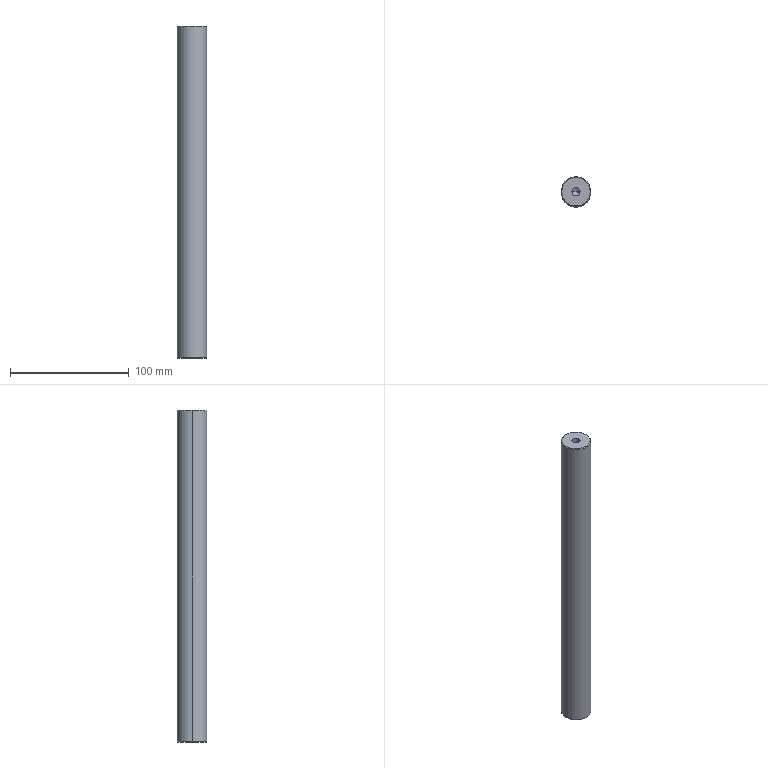Part | SolidWorks | features HoleWzd 2, Chamfer 1, Extrusion 1 | 1 solid | 16 faces | box 25 x 25 x 280 mm | volume 135760 mm3 | cone 8 | cylinder 6 | plane 2 | commonest cylinder face diameters 6.8 x4 25 x2
STEP:
#1=CARTESIAN_POINT('',(-12.,0.,0.));
#2=VERTEX_POINT('',#1);
#3=CARTESIAN_POINT('',(12.,0.,0.));
#4=VERTEX_POINT('',#3);
#5=CARTESIAN_POINT('',(0.,0.,0.));
#6=DIRECTION('',(0.,0.,-1.));
#7=DIRECTION('',(1.,0.,0.));
#8=AXIS2_PLACEMENT_3D('',#5,#6,#7);
#9=CIRCLE('',#8,12.);
#10=EDGE_CURVE('',#2,#4,#9,.T.);
#11=ORIENTED_EDGE('',*,*,#10,.F.);
#12=CARTESIAN_POINT('',(-12.5,0.,0.5));
#13=VERTEX_POINT('',#12);
#14=CARTESIAN_POINT('',(-12.5,0.,0.5));
#15=DIRECTION('',(-0.7071,0.,0.7071));
#16=VECTOR('',#15,1000.);
#17=LINE('',#14,#16);
#18=EDGE_CURVE('',#2,#13,#17,.T.);
#19=ORIENTED_EDGE('',*,*,#18,.T.);
#20=CARTESIAN_POINT('',(12.5,0.,0.5));
#21=VERTEX_POINT('',#20);
#22=CARTESIAN_POINT('',(0.,0.,0.5));
#23=DIRECTION('',(0.,0.,1.));
#24=DIRECTION('',(1.,0.,0.));
#25=AXIS2_PLACEMENT_3D('',#22,#23,#24);
#26=CIRCLE('',#25,12.5);
#27=EDGE_CURVE('',#21,#13,#26,.T.);
#28=ORIENTED_EDGE('',*,*,#27,.F.);
#29=CARTESIAN_POINT('',(12.5,0.,0.5));
#30=DIRECTION('',(0.7071,0.,0.7071));
#31=VECTOR('',#30,1000.);
#32=LINE('',#29,#31);
#33=EDGE_CURVE('',#4,#21,#32,.T.);
#34=ORIENTED_EDGE('',*,*,#33,.F.);
#35=EDGE_LOOP('',(#11,#19,#28,#34));
#36=FACE_OUTER_BOUND('',#35,.T.);
#37=CARTESIAN_POINT('',(0.,0.,0.5));
#38=DIRECTION('',(0.,0.,1.));
#39=DIRECTION('',(1.,0.,0.));
#40=AXIS2_PLACEMENT_3D('',#37,#38,#39);
#41=CONICAL_SURFACE('',#40,12.5,0.7854);
#42=ADVANCED_FACE('',(#36),#41,.T.);
#43=CARTESIAN_POINT('',(12.,0.,280.));
#44=VERTEX_POINT('',#43);
#45=CARTESIAN_POINT('',(-12.,0.,280.));
#46=VERTEX_POINT('',#45);
#47=CARTESIAN_POINT('',(0.,0.,280.));
#48=DIRECTION('',(0.,0.,1.));
#49=DIRECTION('',(1.,0.,0.));
#50=AXIS2_PLACEMENT_3D('',#47,#48,#49);
#51=CIRCLE('',#50,12.);
#52=EDGE_CURVE('',#44,#46,#51,.T.);
#53=ORIENTED_EDGE('',*,*,#52,.F.);
#54=CARTESIAN_POINT('',(12.5,0.,279.5));
#55=VERTEX_POINT('',#54);
#56=CARTESIAN_POINT('',(12.,0.,280.));
#57=DIRECTION('',(0.7071,0.,-0.7071));
#58=VECTOR('',#57,1000.);
#59=LINE('',#56,#58);
#60=EDGE_CURVE('',#44,#55,#59,.T.);
#61=ORIENTED_EDGE('',*,*,#60,.T.);
#62=CARTESIAN_POINT('',(-12.5,0.,279.5));
#63=VERTEX_POINT('',#62);
#64=CARTESIAN_POINT('',(0.,0.,279.5));
#65=DIRECTION('',(0.,0.,-1.));
#66=DIRECTION('',(1.,0.,0.));
#67=AXIS2_PLACEMENT_3D('',#64,#65,#66);
#68=CIRCLE('',#67,12.5);
#69=EDGE_CURVE('',#63,#55,#68,.T.);
#70=ORIENTED_EDGE('',*,*,#69,.F.);
#71=CARTESIAN_POINT('',(-12.,0.,280.));
#72=DIRECTION('',(-0.7071,0.,-0.7071));
#73=VECTOR('',#72,1000.);
#74=LINE('',#71,#73);
#75=EDGE_CURVE('',#46,#63,#74,.T.);
#76=ORIENTED_EDGE('',*,*,#75,.F.);
#77=EDGE_LOOP('',(#53,#61,#70,#76));
#78=FACE_OUTER_BOUND('',#77,.T.);
#79=CARTESIAN_POINT('',(0.,0.,280.));
#80=DIRECTION('',(0.,0.,-1.));
#81=DIRECTION('',(-1.,0.,0.));
#82=AXIS2_PLACEMENT_3D('',#79,#80,#81);
#83=CONICAL_SURFACE('',#82,12.,0.7854);
#84=ADVANCED_FACE('',(#78),#83,.T.);
#85=CARTESIAN_POINT('',(3.4,0.,22.25));
#86=VERTEX_POINT('',#85);
#87=CARTESIAN_POINT('',(-3.4,0.,22.25));
#88=VERTEX_POINT('',#87);
#89=CARTESIAN_POINT('',(0.,0.,22.25));
#90=DIRECTION('',(0.,0.,-1.));
#91=DIRECTION('',(-1.,0.,0.));
#92=AXIS2_PLACEMENT_3D('',#89,#90,#91);
#93=CIRCLE('',#92,3.4);
#94=EDGE_CURVE('',#86,#88,#93,.T.);
#95=ORIENTED_EDGE('',*,*,#94,.F.);
#96=CARTESIAN_POINT('',(3.4,0.,0.));
#97=VERTEX_POINT('',#96);
#98=CARTESIAN_POINT('',(3.4,0.,0.));
#99=DIRECTION('',(0.,0.,-1.));
#100=VECTOR('',#99,1000.);
#101=LINE('',#98,#100);
#102=EDGE_CURVE('',#86,#97,#101,.T.);
#103=ORIENTED_EDGE('',*,*,#102,.T.);
#104=CARTESIAN_POINT('',(-3.4,0.,0.));
#105=VERTEX_POINT('',#104);
#106=CARTESIAN_POINT('',(0.,0.,0.));
#107=DIRECTION('',(0.,0.,-1.));
#108=DIRECTION('',(-1.,0.,0.));
#109=AXIS2_PLACEMENT_3D('',#106,#107,#108);
#110=CIRCLE('',#109,3.4);
#111=EDGE_CURVE('',#97,#105,#110,.T.);
#112=ORIENTED_EDGE('',*,*,#111,.T.);
#113=CARTESIAN_POINT('',(-3.4,0.,0.));
#114=DIRECTION('',(0.,0.,-1.));
#115=VECTOR('',#114,1000.);
#116=LINE('',#113,#115);
#117=EDGE_CURVE('',#88,#105,#116,.T.);
#118=ORIENTED_EDGE('',*,*,#117,.F.);
#119=EDGE_LOOP('',(#95,#103,#112,#118));
#120=FACE_OUTER_BOUND('',#119,.T.);
#121=CARTESIAN_POINT('',(0.,0.,0.));
#122=DIRECTION('',(0.,0.,-1.));
#123=DIRECTION('',(-1.,0.,0.));
#124=AXIS2_PLACEMENT_3D('',#121,#122,#123);
#125=CYLINDRICAL_SURFACE('',#124,3.4);
#126=ADVANCED_FACE('',(#120),#125,.F.);
#127=CARTESIAN_POINT('',(0.,0.,24.293));
#128=VERTEX_POINT('',#127);
#129=CARTESIAN_POINT('',(-3.4,0.,22.25));
#130=DIRECTION('',(-0.8572,0.,-0.515));
#131=VECTOR('',#130,1000.);
#132=LINE('',#129,#131);
#133=EDGE_CURVE('',#128,#88,#132,.T.);
#134=ORIENTED_EDGE('',*,*,#133,.F.);
#135=CARTESIAN_POINT('',(3.4,0.,22.25));
#136=DIRECTION('',(0.8572,0.,-0.515));
#137=VECTOR('',#136,1000.);
#138=LINE('',#135,#137);
#139=EDGE_CURVE('',#128,#86,#138,.T.);
#140=ORIENTED_EDGE('',*,*,#139,.T.);
#141=ORIENTED_EDGE('',*,*,#94,.T.);
#142=EDGE_LOOP('',(#134,#140,#141));
#143=FACE_OUTER_BOUND('',#142,.T.);
#144=CARTESIAN_POINT('',(0.,0.,22.25));
#145=DIRECTION('',(0.,0.,-1.));
#146=DIRECTION('',(-1.,0.,0.));
#147=AXIS2_PLACEMENT_3D('',#144,#145,#146);
#148=CONICAL_SURFACE('',#147,3.4,1.03);
#149=ADVANCED_FACE('',(#143),#148,.F.);
#150=CARTESIAN_POINT('',(-3.4,0.,257.75));
#151=VERTEX_POINT('',#150);
#152=CARTESIAN_POINT('',(3.4,0.,257.75));
#153=VERTEX_POINT('',#152);
#154=CARTESIAN_POINT('',(0.,0.,257.75));
#155=DIRECTION('',(0.,0.,1.));
#156=DIRECTION('',(1.,0.,0.));
#157=AXIS2_PLACEMENT_3D('',#154,#155,#156);
#158=CIRCLE('',#157,3.4);
#159=EDGE_CURVE('',#151,#153,#158,.T.);
#160=ORIENTED_EDGE('',*,*,#159,.F.);
#161=CARTESIAN_POINT('',(-3.4,0.,280.));
#162=VERTEX_POINT('',#161);
#163=CARTESIAN_POINT('',(-3.4,0.,280.));
#164=DIRECTION('',(0.,0.,1.));
#165=VECTOR('',#164,1000.);
#166=LINE('',#163,#165);
#167=EDGE_CURVE('',#151,#162,#166,.T.);
#168=ORIENTED_EDGE('',*,*,#167,.T.);
#169=CARTESIAN_POINT('',(3.4,0.,280.));
#170=VERTEX_POINT('',#169);
#171=CARTESIAN_POINT('',(0.,0.,280.));
#172=DIRECTION('',(0.,0.,1.));
#173=DIRECTION('',(1.,0.,0.));
#174=AXIS2_PLACEMENT_3D('',#171,#172,#173);
#175=CIRCLE('',#174,3.4);
#176=EDGE_CURVE('',#162,#170,#175,.T.);
#177=ORIENTED_EDGE('',*,*,#176,.T.);
#178=CARTESIAN_POINT('',(3.4,0.,280.));
#179=DIRECTION('',(0.,0.,1.));
#180=VECTOR('',#179,1000.);
#181=LINE('',#178,#180);
#182=EDGE_CURVE('',#153,#170,#181,.T.);
#183=ORIENTED_EDGE('',*,*,#182,.F.);
#184=EDGE_LOOP('',(#160,#168,#177,#183));
#185=FACE_OUTER_BOUND('',#184,.T.);
#186=CARTESIAN_POINT('',(0.,0.,280.));
#187=DIRECTION('',(0.,0.,1.));
#188=DIRECTION('',(1.,0.,0.));
#189=AXIS2_PLACEMENT_3D('',#186,#187,#188);
#190=CYLINDRICAL_SURFACE('',#189,3.4);
#191=ADVANCED_FACE('',(#185),#190,.F.);
#192=CARTESIAN_POINT('',(0.,0.,255.707));
#193=VERTEX_POINT('',#192);
#194=CARTESIAN_POINT('',(3.4,0.,257.75));
#195=DIRECTION('',(0.8572,0.,0.515));
#196=VECTOR('',#195,1000.);
#197=LINE('',#194,#196);
#198=EDGE_CURVE('',#193,#153,#197,.T.);
#199=ORIENTED_EDGE('',*,*,#198,.F.);
#200=CARTESIAN_POINT('',(-3.4,0.,257.75));
#201=DIRECTION('',(-0.8572,0.,0.515));
#202=VECTOR('',#201,1000.);
#203=LINE('',#200,#202);
#204=EDGE_CURVE('',#193,#151,#203,.T.);
#205=ORIENTED_EDGE('',*,*,#204,.T.);
#206=ORIENTED_EDGE('',*,*,#159,.T.);
#207=EDGE_LOOP('',(#199,#205,#206));
#208=FACE_OUTER_BOUND('',#207,.T.);
#209=CARTESIAN_POINT('',(0.,0.,257.75));
#210=DIRECTION('',(0.,0.,1.));
#211=DIRECTION('',(1.,0.,0.));
#212=AXIS2_PLACEMENT_3D('',#209,#210,#211);
#213=CONICAL_SURFACE('',#212,3.4,1.03);
#214=ADVANCED_FACE('',(#208),#213,.F.);
#215=ORIENTED_EDGE('',*,*,#69,.T.);
#216=CARTESIAN_POINT('',(12.5,0.,280.));
#217=DIRECTION('',(0.,0.,-1.));
#218=VECTOR('',#217,1000.);
#219=LINE('',#216,#218);
#220=EDGE_CURVE('',#55,#21,#219,.T.);
#221=ORIENTED_EDGE('',*,*,#220,.T.);
#222=ORIENTED_EDGE('',*,*,#27,.T.);
#223=CARTESIAN_POINT('',(-12.5,0.,280.));
#224=DIRECTION('',(0.,0.,-1.));
#225=VECTOR('',#224,1000.);
#226=LINE('',#223,#225);
#227=EDGE_CURVE('',#63,#13,#226,.T.);
#228=ORIENTED_EDGE('',*,*,#227,.F.);
#229=EDGE_LOOP('',(#215,#221,#222,#228));
#230=FACE_OUTER_BOUND('',#229,.T.);
#231=CARTESIAN_POINT('',(0.,0.,280.));
#232=DIRECTION('',(0.,0.,-1.));
#233=DIRECTION('',(-1.,0.,0.));
#234=AXIS2_PLACEMENT_3D('',#231,#232,#233);
#235=CYLINDRICAL_SURFACE('',#234,12.5);
#236=ADVANCED_FACE('',(#230),#235,.T.);
#237=ORIENTED_EDGE('',*,*,#220,.F.);
#238=CARTESIAN_POINT('',(0.,0.,279.5));
#239=DIRECTION('',(0.,0.,-1.));
#240=DIRECTION('',(1.,0.,0.));
#241=AXIS2_PLACEMENT_3D('',#238,#239,#240);
#242=CIRCLE('',#241,12.5);
#243=EDGE_CURVE('',#55,#63,#242,.T.);
#244=ORIENTED_EDGE('',*,*,#243,.T.);
#245=ORIENTED_EDGE('',*,*,#227,.T.);
#246=CARTESIAN_POINT('',(0.,0.,0.5));
#247=DIRECTION('',(0.,0.,1.));
#248=DIRECTION('',(1.,0.,0.));
#249=AXIS2_PLACEMENT_3D('',#246,#247,#248);
#250=CIRCLE('',#249,12.5);
#251=EDGE_CURVE('',#13,#21,#250,.T.);
#252=ORIENTED_EDGE('',*,*,#251,.T.);
#253=EDGE_LOOP('',(#237,#244,#245,#252));
#254=FACE_OUTER_BOUND('',#253,.T.);
#255=CARTESIAN_POINT('',(0.,0.,280.));
#256=DIRECTION('',(0.,0.,-1.));
#257=DIRECTION('',(-1.,0.,0.));
#258=AXIS2_PLACEMENT_3D('',#255,#256,#257);
#259=CYLINDRICAL_SURFACE('',#258,12.5);
#260=ADVANCED_FACE('',(#254),#259,.T.);
#261=CARTESIAN_POINT('',(0.,0.,280.));
#262=DIRECTION('',(0.,0.,1.));
#263=DIRECTION('',(1.,0.,0.));
#264=AXIS2_PLACEMENT_3D('',#261,#262,#263);
#265=CIRCLE('',#264,12.);
#266=EDGE_CURVE('',#46,#44,#265,.T.);
#267=ORIENTED_EDGE('',*,*,#266,.T.);
#268=ORIENTED_EDGE('',*,*,#52,.T.);
#269=EDGE_LOOP('',(#267,#268));
#270=FACE_OUTER_BOUND('',#269,.T.);
#271=CARTESIAN_POINT('',(0.,0.,280.));
#272=DIRECTION('',(0.,0.,1.));
#273=DIRECTION('',(1.,0.,0.));
#274=AXIS2_PLACEMENT_3D('',#271,#272,#273);
#275=CIRCLE('',#274,3.4);
#276=EDGE_CURVE('',#170,#162,#275,.T.);
#277=ORIENTED_EDGE('',*,*,#276,.F.);
#278=ORIENTED_EDGE('',*,*,#176,.F.);
#279=EDGE_LOOP('',(#277,#278));
#280=FACE_BOUND('',#279,.T.);
#281=CARTESIAN_POINT('',(0.,0.,280.));
#282=DIRECTION('',(0.,0.,1.));
#283=DIRECTION('',(1.,0.,0.));
#284=AXIS2_PLACEMENT_3D('',#281,#282,#283);
#285=PLANE('',#284);
#286=ADVANCED_FACE('',(#270,#280),#285,.T.);
#287=CARTESIAN_POINT('',(0.,0.,0.));
#288=DIRECTION('',(0.,0.,-1.));
#289=DIRECTION('',(1.,0.,0.));
#290=AXIS2_PLACEMENT_3D('',#287,#288,#289);
#291=CIRCLE('',#290,12.);
#292=EDGE_CURVE('',#4,#2,#291,.T.);
#293=ORIENTED_EDGE('',*,*,#292,.T.);
#294=ORIENTED_EDGE('',*,*,#10,.T.);
#295=EDGE_LOOP('',(#293,#294));
#296=FACE_OUTER_BOUND('',#295,.T.);
#297=CARTESIAN_POINT('',(0.,0.,0.));
#298=DIRECTION('',(0.,0.,-1.));
#299=DIRECTION('',(-1.,0.,0.));
#300=AXIS2_PLACEMENT_3D('',#297,#298,#299);
#301=CIRCLE('',#300,3.4);
#302=EDGE_CURVE('',#105,#97,#301,.T.);
#303=ORIENTED_EDGE('',*,*,#302,.F.);
#304=ORIENTED_EDGE('',*,*,#111,.F.);
#305=EDGE_LOOP('',(#303,#304));
#306=FACE_BOUND('',#305,.T.);
#307=CARTESIAN_POINT('',(0.,0.,0.));
#308=DIRECTION('',(0.,0.,1.));
#309=DIRECTION('',(1.,0.,0.));
#310=AXIS2_PLACEMENT_3D('',#307,#308,#309);
#311=PLANE('',#310);
#312=ADVANCED_FACE('',(#296,#306),#311,.F.);
#313=ORIENTED_EDGE('',*,*,#204,.F.);
#314=ORIENTED_EDGE('',*,*,#198,.T.);
#315=CARTESIAN_POINT('',(0.,0.,257.75));
#316=DIRECTION('',(0.,0.,1.));
#317=DIRECTION('',(1.,0.,0.));
#318=AXIS2_PLACEMENT_3D('',#315,#316,#317);
#319=CIRCLE('',#318,3.4);
#320=EDGE_CURVE('',#153,#151,#319,.T.);
#321=ORIENTED_EDGE('',*,*,#320,.T.);
#322=EDGE_LOOP('',(#313,#314,#321));
#323=FACE_OUTER_BOUND('',#322,.T.);
#324=CARTESIAN_POINT('',(0.,0.,257.75));
#325=DIRECTION('',(0.,0.,1.));
#326=DIRECTION('',(1.,0.,0.));
#327=AXIS2_PLACEMENT_3D('',#324,#325,#326);
#328=CONICAL_SURFACE('',#327,3.4,1.03);
#329=ADVANCED_FACE('',(#323),#328,.F.);
#330=ORIENTED_EDGE('',*,*,#167,.F.);
#331=ORIENTED_EDGE('',*,*,#320,.F.);
#332=ORIENTED_EDGE('',*,*,#182,.T.);
#333=ORIENTED_EDGE('',*,*,#276,.T.);
#334=EDGE_LOOP('',(#330,#331,#332,#333));
#335=FACE_OUTER_BOUND('',#334,.T.);
#336=CARTESIAN_POINT('',(0.,0.,280.));
#337=DIRECTION('',(0.,0.,1.));
#338=DIRECTION('',(1.,0.,0.));
#339=AXIS2_PLACEMENT_3D('',#336,#337,#338);
#340=CYLINDRICAL_SURFACE('',#339,3.4);
#341=ADVANCED_FACE('',(#335),#340,.F.);
#342=ORIENTED_EDGE('',*,*,#139,.F.);
#343=ORIENTED_EDGE('',*,*,#133,.T.);
#344=CARTESIAN_POINT('',(0.,0.,22.25));
#345=DIRECTION('',(0.,0.,-1.));
#346=DIRECTION('',(-1.,0.,0.));
#347=AXIS2_PLACEMENT_3D('',#344,#345,#346);
#348=CIRCLE('',#347,3.4);
#349=EDGE_CURVE('',#88,#86,#348,.T.);
#350=ORIENTED_EDGE('',*,*,#349,.T.);
#351=EDGE_LOOP('',(#342,#343,#350));
#352=FACE_OUTER_BOUND('',#351,.T.);
#353=CARTESIAN_POINT('',(0.,0.,22.25));
#354=DIRECTION('',(0.,0.,-1.));
#355=DIRECTION('',(-1.,0.,0.));
#356=AXIS2_PLACEMENT_3D('',#353,#354,#355);
#357=CONICAL_SURFACE('',#356,3.4,1.03);
#358=ADVANCED_FACE('',(#352),#357,.F.);
#359=ORIENTED_EDGE('',*,*,#102,.F.);
#360=ORIENTED_EDGE('',*,*,#349,.F.);
#361=ORIENTED_EDGE('',*,*,#117,.T.);
#362=ORIENTED_EDGE('',*,*,#302,.T.);
#363=EDGE_LOOP('',(#359,#360,#361,#362));
#364=FACE_OUTER_BOUND('',#363,.T.);
#365=CARTESIAN_POINT('',(0.,0.,0.));
#366=DIRECTION('',(0.,0.,-1.));
#367=DIRECTION('',(-1.,0.,0.));
#368=AXIS2_PLACEMENT_3D('',#365,#366,#367);
#369=CYLINDRICAL_SURFACE('',#368,3.4);
#370=ADVANCED_FACE('',(#364),#369,.F.);
#371=ORIENTED_EDGE('',*,*,#60,.F.);
#372=ORIENTED_EDGE('',*,*,#266,.F.);
#373=ORIENTED_EDGE('',*,*,#75,.T.);
#374=ORIENTED_EDGE('',*,*,#243,.F.);
#375=EDGE_LOOP('',(#371,#372,#373,#374));
#376=FACE_OUTER_BOUND('',#375,.T.);
#377=CARTESIAN_POINT('',(0.,0.,280.));
#378=DIRECTION('',(0.,0.,-1.));
#379=DIRECTION('',(-1.,0.,0.));
#380=AXIS2_PLACEMENT_3D('',#377,#378,#379);
#381=CONICAL_SURFACE('',#380,12.,0.7854);
#382=ADVANCED_FACE('',(#376),#381,.T.);
#383=ORIENTED_EDGE('',*,*,#18,.F.);
#384=ORIENTED_EDGE('',*,*,#292,.F.);
#385=ORIENTED_EDGE('',*,*,#33,.T.);
#386=ORIENTED_EDGE('',*,*,#251,.F.);
#387=EDGE_LOOP('',(#383,#384,#385,#386));
#388=FACE_OUTER_BOUND('',#387,.T.);
#389=CARTESIAN_POINT('',(0.,0.,0.5));
#390=DIRECTION('',(0.,0.,1.));
#391=DIRECTION('',(1.,0.,0.));
#392=AXIS2_PLACEMENT_3D('',#389,#390,#391);
#393=CONICAL_SURFACE('',#392,12.5,0.7854);
#394=ADVANCED_FACE('',(#388),#393,.T.);
#395=CLOSED_SHELL('',(#42,#84,#126,#149,#191,#214,#236,#260,#286,#312,#329,#341,#358,#370,#382,#394));
#396=MANIFOLD_SOLID_BREP('',#395);
#397=CARTESIAN_POINT('',(0.,0.,0.));
#398=DIRECTION('',(0.,0.,1.));
#399=DIRECTION('',(1.,0.,0.));
#400=AXIS2_PLACEMENT_3D('',#397,#398,#399);
#401=(LENGTH_UNIT()NAMED_UNIT(*)SI_UNIT(.MILLI.,.METRE.));
#402=UNCERTAINTY_MEASURE_WITH_UNIT(LENGTH_MEASURE(0.00001),#401,'','');
#403=(NAMED_UNIT(*)PLANE_ANGLE_UNIT()SI_UNIT($,.RADIAN.));
#404=(NAMED_UNIT(*)SI_UNIT($,.STERADIAN.)SOLID_ANGLE_UNIT());
#405=(GEOMETRIC_REPRESENTATION_CONTEXT(3)GLOBAL_UNCERTAINTY_ASSIGNED_CONTEXT((#402))GLOBAL_UNIT_ASSIGNED_CONTEXT((#401,#403,#404))REPRESENTATION_CONTEXT('',''));
#406=ADVANCED_BREP_SHAPE_REPRESENTATION('',(#396,#400),#405);